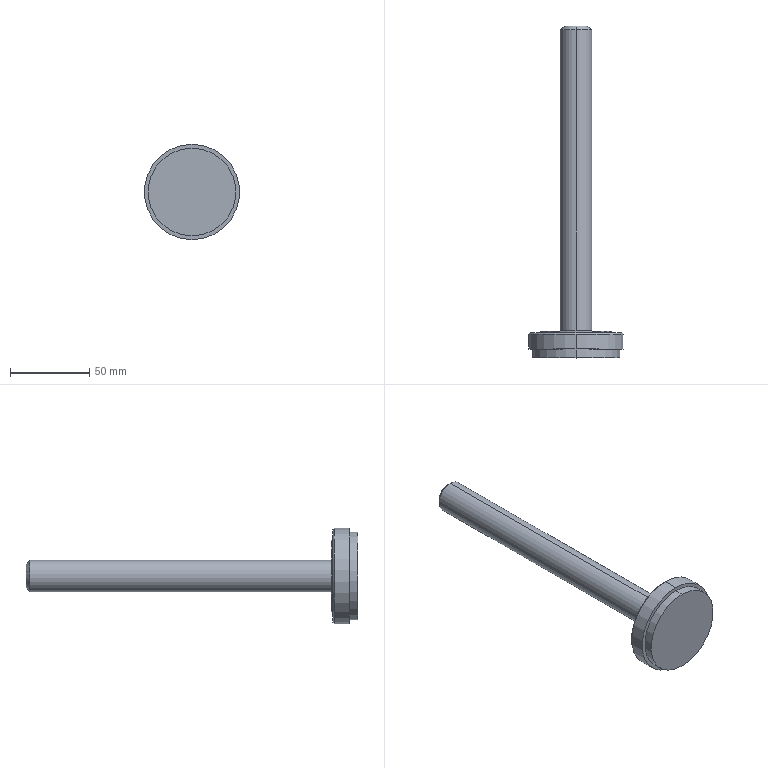Part | STEP file | SceondD-B3-20-180 | 1 solid | 17 faces | box 60.3 x 210 x 60.3 mm | volume 105197 mm3 | cylinder 8 | plane 5 | cone 4 | commonest cylinder face diameters 20 x2 45 x2 55.5 x2 60.3 x2
STEP:
#1=CARTESIAN_POINT('',(0.,0.,27.75));
#2=VERTEX_POINT('',#1);
#3=CARTESIAN_POINT('',(0.,0.,-27.75));
#4=VERTEX_POINT('',#3);
#5=CARTESIAN_POINT('',(0.,0.,0.));
#6=DIRECTION('',(0.,1.,0.));
#7=DIRECTION('',(0.,0.,1.));
#8=AXIS2_PLACEMENT_3D('',#5,#6,#7);
#9=CIRCLE('',#8,27.75);
#10=EDGE_CURVE('',#2,#4,#9,.T.);
#11=ORIENTED_EDGE('',*,*,#10,.T.);
#12=CARTESIAN_POINT('',(0.,5.6,-27.75));
#13=VERTEX_POINT('',#12);
#14=CARTESIAN_POINT('',(0.,210.,-27.75));
#15=DIRECTION('',(0.,1.,0.));
#16=VECTOR('',#15,1000.);
#17=LINE('',#14,#16);
#18=EDGE_CURVE('',#4,#13,#17,.T.);
#19=ORIENTED_EDGE('',*,*,#18,.T.);
#20=CARTESIAN_POINT('',(0.,5.6,27.75));
#21=VERTEX_POINT('',#20);
#22=CARTESIAN_POINT('',(0.,5.6,0.));
#23=DIRECTION('',(0.,1.,0.));
#24=DIRECTION('',(0.,0.,1.));
#25=AXIS2_PLACEMENT_3D('',#22,#23,#24);
#26=CIRCLE('',#25,27.75);
#27=EDGE_CURVE('',#21,#13,#26,.T.);
#28=ORIENTED_EDGE('',*,*,#27,.F.);
#29=CARTESIAN_POINT('',(0.,210.,27.75));
#30=DIRECTION('',(0.,1.,0.));
#31=VECTOR('',#30,1000.);
#32=LINE('',#29,#31);
#33=EDGE_CURVE('',#2,#21,#32,.T.);
#34=ORIENTED_EDGE('',*,*,#33,.F.);
#35=EDGE_LOOP('',(#11,#19,#28,#34));
#36=FACE_OUTER_BOUND('',#35,.T.);
#37=CARTESIAN_POINT('',(0.,210.,0.));
#38=DIRECTION('',(0.,1.,0.));
#39=DIRECTION('',(0.,0.,1.));
#40=AXIS2_PLACEMENT_3D('',#37,#38,#39);
#41=CYLINDRICAL_SURFACE('',#40,27.75);
#42=ADVANCED_FACE('',(#36),#41,.T.);
#43=CARTESIAN_POINT('',(0.,5.6,30.15));
#44=VERTEX_POINT('',#43);
#45=CARTESIAN_POINT('',(0.,5.6,-30.15));
#46=VERTEX_POINT('',#45);
#47=CARTESIAN_POINT('',(0.,5.6,0.));
#48=DIRECTION('',(0.,1.,0.));
#49=DIRECTION('',(0.,0.,1.));
#50=AXIS2_PLACEMENT_3D('',#47,#48,#49);
#51=CIRCLE('',#50,30.15);
#52=EDGE_CURVE('',#44,#46,#51,.T.);
#53=ORIENTED_EDGE('',*,*,#52,.T.);
#54=CARTESIAN_POINT('',(0.,15.,-30.15));
#55=VERTEX_POINT('',#54);
#56=CARTESIAN_POINT('',(0.,210.,-30.15));
#57=DIRECTION('',(0.,1.,0.));
#58=VECTOR('',#57,1000.);
#59=LINE('',#56,#58);
#60=EDGE_CURVE('',#46,#55,#59,.T.);
#61=ORIENTED_EDGE('',*,*,#60,.T.);
#62=CARTESIAN_POINT('',(0.,15.,30.15));
#63=VERTEX_POINT('',#62);
#64=CARTESIAN_POINT('',(0.,15.,0.));
#65=DIRECTION('',(0.,1.,0.));
#66=DIRECTION('',(0.,0.,1.));
#67=AXIS2_PLACEMENT_3D('',#64,#65,#66);
#68=CIRCLE('',#67,30.15);
#69=EDGE_CURVE('',#63,#55,#68,.T.);
#70=ORIENTED_EDGE('',*,*,#69,.F.);
#71=CARTESIAN_POINT('',(0.,210.,30.15));
#72=DIRECTION('',(0.,1.,0.));
#73=VECTOR('',#72,1000.);
#74=LINE('',#71,#73);
#75=EDGE_CURVE('',#44,#63,#74,.T.);
#76=ORIENTED_EDGE('',*,*,#75,.F.);
#77=EDGE_LOOP('',(#53,#61,#70,#76));
#78=FACE_OUTER_BOUND('',#77,.T.);
#79=CARTESIAN_POINT('',(0.,210.,0.));
#80=DIRECTION('',(0.,1.,0.));
#81=DIRECTION('',(0.,0.,1.));
#82=AXIS2_PLACEMENT_3D('',#79,#80,#81);
#83=CYLINDRICAL_SURFACE('',#82,30.15);
#84=ADVANCED_FACE('',(#78),#83,.T.);
#85=CARTESIAN_POINT('',(0.,16.,29.15));
#86=VERTEX_POINT('',#85);
#87=CARTESIAN_POINT('',(0.,16.,-29.15));
#88=VERTEX_POINT('',#87);
#89=CARTESIAN_POINT('',(0.,16.,0.));
#90=DIRECTION('',(0.,1.,0.));
#91=DIRECTION('',(0.,0.,1.));
#92=AXIS2_PLACEMENT_3D('',#89,#90,#91);
#93=CIRCLE('',#92,29.15);
#94=EDGE_CURVE('',#86,#88,#93,.T.);
#95=ORIENTED_EDGE('',*,*,#94,.F.);
#96=CARTESIAN_POINT('',(0.,16.,29.15));
#97=DIRECTION('',(0.,-0.7071,0.7071));
#98=VECTOR('',#97,1000.);
#99=LINE('',#96,#98);
#100=EDGE_CURVE('',#86,#63,#99,.T.);
#101=ORIENTED_EDGE('',*,*,#100,.T.);
#102=ORIENTED_EDGE('',*,*,#69,.T.);
#103=CARTESIAN_POINT('',(0.,16.,-29.15));
#104=DIRECTION('',(0.,-0.7071,-0.7071));
#105=VECTOR('',#104,1000.);
#106=LINE('',#103,#105);
#107=EDGE_CURVE('',#88,#55,#106,.T.);
#108=ORIENTED_EDGE('',*,*,#107,.F.);
#109=EDGE_LOOP('',(#95,#101,#102,#108));
#110=FACE_OUTER_BOUND('',#109,.T.);
#111=CARTESIAN_POINT('',(0.,16.,0.));
#112=DIRECTION('',(0.,-1.,0.));
#113=DIRECTION('',(0.,0.,-1.));
#114=AXIS2_PLACEMENT_3D('',#111,#112,#113);
#115=CONICAL_SURFACE('',#114,29.15,0.7854);
#116=ADVANCED_FACE('',(#110),#115,.T.);
#117=CARTESIAN_POINT('',(0.,16.,22.5));
#118=VERTEX_POINT('',#117);
#119=CARTESIAN_POINT('',(0.,16.,-22.5));
#120=VERTEX_POINT('',#119);
#121=CARTESIAN_POINT('',(0.,16.,0.));
#122=DIRECTION('',(0.,1.,0.));
#123=DIRECTION('',(0.,0.,1.));
#124=AXIS2_PLACEMENT_3D('',#121,#122,#123);
#125=CIRCLE('',#124,22.5);
#126=EDGE_CURVE('',#118,#120,#125,.T.);
#127=ORIENTED_EDGE('',*,*,#126,.T.);
#128=CARTESIAN_POINT('',(0.,17.,-22.5));
#129=VERTEX_POINT('',#128);
#130=CARTESIAN_POINT('',(0.,210.,-22.5));
#131=DIRECTION('',(0.,1.,0.));
#132=VECTOR('',#131,1000.);
#133=LINE('',#130,#132);
#134=EDGE_CURVE('',#120,#129,#133,.T.);
#135=ORIENTED_EDGE('',*,*,#134,.T.);
#136=CARTESIAN_POINT('',(0.,17.,22.5));
#137=VERTEX_POINT('',#136);
#138=CARTESIAN_POINT('',(0.,17.,0.));
#139=DIRECTION('',(0.,1.,0.));
#140=DIRECTION('',(0.,0.,1.));
#141=AXIS2_PLACEMENT_3D('',#138,#139,#140);
#142=CIRCLE('',#141,22.5);
#143=EDGE_CURVE('',#137,#129,#142,.T.);
#144=ORIENTED_EDGE('',*,*,#143,.F.);
#145=CARTESIAN_POINT('',(0.,210.,22.5));
#146=DIRECTION('',(0.,1.,0.));
#147=VECTOR('',#146,1000.);
#148=LINE('',#145,#147);
#149=EDGE_CURVE('',#118,#137,#148,.T.);
#150=ORIENTED_EDGE('',*,*,#149,.F.);
#151=EDGE_LOOP('',(#127,#135,#144,#150));
#152=FACE_OUTER_BOUND('',#151,.T.);
#153=CARTESIAN_POINT('',(0.,210.,0.));
#154=DIRECTION('',(0.,1.,0.));
#155=DIRECTION('',(0.,0.,1.));
#156=AXIS2_PLACEMENT_3D('',#153,#154,#155);
#157=CYLINDRICAL_SURFACE('',#156,22.5);
#158=ADVANCED_FACE('',(#152),#157,.T.);
#159=CARTESIAN_POINT('',(0.,17.,10.));
#160=VERTEX_POINT('',#159);
#161=CARTESIAN_POINT('',(0.,17.,-10.));
#162=VERTEX_POINT('',#161);
#163=CARTESIAN_POINT('',(0.,17.,0.));
#164=DIRECTION('',(0.,1.,0.));
#165=DIRECTION('',(0.,0.,1.));
#166=AXIS2_PLACEMENT_3D('',#163,#164,#165);
#167=CIRCLE('',#166,10.);
#168=EDGE_CURVE('',#160,#162,#167,.T.);
#169=ORIENTED_EDGE('',*,*,#168,.T.);
#170=CARTESIAN_POINT('',(0.,207.5,-10.));
#171=VERTEX_POINT('',#170);
#172=CARTESIAN_POINT('',(0.,210.,-10.));
#173=DIRECTION('',(0.,1.,0.));
#174=VECTOR('',#173,1000.);
#175=LINE('',#172,#174);
#176=EDGE_CURVE('',#162,#171,#175,.T.);
#177=ORIENTED_EDGE('',*,*,#176,.T.);
#178=CARTESIAN_POINT('',(0.,207.5,10.));
#179=VERTEX_POINT('',#178);
#180=CARTESIAN_POINT('',(0.,207.5,0.));
#181=DIRECTION('',(0.,1.,0.));
#182=DIRECTION('',(0.,0.,1.));
#183=AXIS2_PLACEMENT_3D('',#180,#181,#182);
#184=CIRCLE('',#183,10.);
#185=EDGE_CURVE('',#179,#171,#184,.T.);
#186=ORIENTED_EDGE('',*,*,#185,.F.);
#187=CARTESIAN_POINT('',(0.,210.,10.));
#188=DIRECTION('',(0.,1.,0.));
#189=VECTOR('',#188,1000.);
#190=LINE('',#187,#189);
#191=EDGE_CURVE('',#160,#179,#190,.T.);
#192=ORIENTED_EDGE('',*,*,#191,.F.);
#193=EDGE_LOOP('',(#169,#177,#186,#192));
#194=FACE_OUTER_BOUND('',#193,.T.);
#195=CARTESIAN_POINT('',(0.,210.,0.));
#196=DIRECTION('',(0.,1.,0.));
#197=DIRECTION('',(0.,0.,1.));
#198=AXIS2_PLACEMENT_3D('',#195,#196,#197);
#199=CYLINDRICAL_SURFACE('',#198,10.);
#200=ADVANCED_FACE('',(#194),#199,.T.);
#201=CARTESIAN_POINT('',(0.,210.,7.5));
#202=VERTEX_POINT('',#201);
#203=CARTESIAN_POINT('',(0.,210.,-7.5));
#204=VERTEX_POINT('',#203);
#205=CARTESIAN_POINT('',(0.,210.,0.));
#206=DIRECTION('',(0.,1.,0.));
#207=DIRECTION('',(0.,0.,1.));
#208=AXIS2_PLACEMENT_3D('',#205,#206,#207);
#209=CIRCLE('',#208,7.5);
#210=EDGE_CURVE('',#202,#204,#209,.T.);
#211=ORIENTED_EDGE('',*,*,#210,.F.);
#212=CARTESIAN_POINT('',(0.,210.,7.5));
#213=DIRECTION('',(0.,-0.7071,0.7071));
#214=VECTOR('',#213,1000.);
#215=LINE('',#212,#214);
#216=EDGE_CURVE('',#202,#179,#215,.T.);
#217=ORIENTED_EDGE('',*,*,#216,.T.);
#218=ORIENTED_EDGE('',*,*,#185,.T.);
#219=CARTESIAN_POINT('',(0.,210.,-7.5));
#220=DIRECTION('',(0.,-0.7071,-0.7071));
#221=VECTOR('',#220,1000.);
#222=LINE('',#219,#221);
#223=EDGE_CURVE('',#204,#171,#222,.T.);
#224=ORIENTED_EDGE('',*,*,#223,.F.);
#225=EDGE_LOOP('',(#211,#217,#218,#224));
#226=FACE_OUTER_BOUND('',#225,.T.);
#227=CARTESIAN_POINT('',(0.,210.,0.));
#228=DIRECTION('',(0.,-1.,0.));
#229=DIRECTION('',(0.,0.,-1.));
#230=AXIS2_PLACEMENT_3D('',#227,#228,#229);
#231=CONICAL_SURFACE('',#230,7.5,0.7854);
#232=ADVANCED_FACE('',(#226),#231,.T.);
#233=ORIENTED_EDGE('',*,*,#216,.F.);
#234=CARTESIAN_POINT('',(0.,210.,0.));
#235=DIRECTION('',(0.,1.,0.));
#236=DIRECTION('',(0.,0.,1.));
#237=AXIS2_PLACEMENT_3D('',#234,#235,#236);
#238=CIRCLE('',#237,7.5);
#239=EDGE_CURVE('',#204,#202,#238,.T.);
#240=ORIENTED_EDGE('',*,*,#239,.F.);
#241=ORIENTED_EDGE('',*,*,#223,.T.);
#242=CARTESIAN_POINT('',(0.,207.5,0.));
#243=DIRECTION('',(0.,1.,0.));
#244=DIRECTION('',(0.,0.,1.));
#245=AXIS2_PLACEMENT_3D('',#242,#243,#244);
#246=CIRCLE('',#245,10.);
#247=EDGE_CURVE('',#171,#179,#246,.T.);
#248=ORIENTED_EDGE('',*,*,#247,.T.);
#249=EDGE_LOOP('',(#233,#240,#241,#248));
#250=FACE_OUTER_BOUND('',#249,.T.);
#251=CARTESIAN_POINT('',(0.,210.,0.));
#252=DIRECTION('',(0.,-1.,0.));
#253=DIRECTION('',(0.,0.,-1.));
#254=AXIS2_PLACEMENT_3D('',#251,#252,#253);
#255=CONICAL_SURFACE('',#254,7.5,0.7854);
#256=ADVANCED_FACE('',(#250),#255,.T.);
#257=ORIENTED_EDGE('',*,*,#176,.F.);
#258=CARTESIAN_POINT('',(0.,17.,0.));
#259=DIRECTION('',(0.,1.,0.));
#260=DIRECTION('',(0.,0.,1.));
#261=AXIS2_PLACEMENT_3D('',#258,#259,#260);
#262=CIRCLE('',#261,10.);
#263=EDGE_CURVE('',#162,#160,#262,.T.);
#264=ORIENTED_EDGE('',*,*,#263,.T.);
#265=ORIENTED_EDGE('',*,*,#191,.T.);
#266=ORIENTED_EDGE('',*,*,#247,.F.);
#267=EDGE_LOOP('',(#257,#264,#265,#266));
#268=FACE_OUTER_BOUND('',#267,.T.);
#269=CARTESIAN_POINT('',(0.,210.,0.));
#270=DIRECTION('',(0.,1.,0.));
#271=DIRECTION('',(0.,0.,1.));
#272=AXIS2_PLACEMENT_3D('',#269,#270,#271);
#273=CYLINDRICAL_SURFACE('',#272,10.);
#274=ADVANCED_FACE('',(#268),#273,.T.);
#275=ORIENTED_EDGE('',*,*,#143,.T.);
#276=CARTESIAN_POINT('',(0.,17.,0.));
#277=DIRECTION('',(0.,1.,0.));
#278=DIRECTION('',(0.,0.,1.));
#279=AXIS2_PLACEMENT_3D('',#276,#277,#278);
#280=CIRCLE('',#279,22.5);
#281=EDGE_CURVE('',#129,#137,#280,.T.);
#282=ORIENTED_EDGE('',*,*,#281,.T.);
#283=EDGE_LOOP('',(#275,#282));
#284=FACE_OUTER_BOUND('',#283,.T.);
#285=ORIENTED_EDGE('',*,*,#168,.F.);
#286=ORIENTED_EDGE('',*,*,#263,.F.);
#287=EDGE_LOOP('',(#285,#286));
#288=FACE_BOUND('',#287,.T.);
#289=CARTESIAN_POINT('',(-22.5,17.,0.));
#290=DIRECTION('',(0.,1.,0.));
#291=DIRECTION('',(0.,0.,1.));
#292=AXIS2_PLACEMENT_3D('',#289,#290,#291);
#293=PLANE('',#292);
#294=ADVANCED_FACE('',(#284,#288),#293,.T.);
#295=ORIENTED_EDGE('',*,*,#134,.F.);
#296=CARTESIAN_POINT('',(0.,16.,0.));
#297=DIRECTION('',(0.,1.,0.));
#298=DIRECTION('',(0.,0.,1.));
#299=AXIS2_PLACEMENT_3D('',#296,#297,#298);
#300=CIRCLE('',#299,22.5);
#301=EDGE_CURVE('',#120,#118,#300,.T.);
#302=ORIENTED_EDGE('',*,*,#301,.T.);
#303=ORIENTED_EDGE('',*,*,#149,.T.);
#304=ORIENTED_EDGE('',*,*,#281,.F.);
#305=EDGE_LOOP('',(#295,#302,#303,#304));
#306=FACE_OUTER_BOUND('',#305,.T.);
#307=CARTESIAN_POINT('',(0.,210.,0.));
#308=DIRECTION('',(0.,1.,0.));
#309=DIRECTION('',(0.,0.,1.));
#310=AXIS2_PLACEMENT_3D('',#307,#308,#309);
#311=CYLINDRICAL_SURFACE('',#310,22.5);
#312=ADVANCED_FACE('',(#306),#311,.T.);
#313=CARTESIAN_POINT('',(0.,16.,0.));
#314=DIRECTION('',(0.,1.,0.));
#315=DIRECTION('',(0.,0.,1.));
#316=AXIS2_PLACEMENT_3D('',#313,#314,#315);
#317=CIRCLE('',#316,29.15);
#318=EDGE_CURVE('',#88,#86,#317,.T.);
#319=ORIENTED_EDGE('',*,*,#318,.T.);
#320=ORIENTED_EDGE('',*,*,#94,.T.);
#321=EDGE_LOOP('',(#319,#320));
#322=FACE_OUTER_BOUND('',#321,.T.);
#323=ORIENTED_EDGE('',*,*,#126,.F.);
#324=ORIENTED_EDGE('',*,*,#301,.F.);
#325=EDGE_LOOP('',(#323,#324));
#326=FACE_BOUND('',#325,.T.);
#327=CARTESIAN_POINT('',(-29.15,16.,0.));
#328=DIRECTION('',(0.,1.,0.));
#329=DIRECTION('',(0.,0.,1.));
#330=AXIS2_PLACEMENT_3D('',#327,#328,#329);
#331=PLANE('',#330);
#332=ADVANCED_FACE('',(#322,#326),#331,.T.);
#333=ORIENTED_EDGE('',*,*,#100,.F.);
#334=ORIENTED_EDGE('',*,*,#318,.F.);
#335=ORIENTED_EDGE('',*,*,#107,.T.);
#336=CARTESIAN_POINT('',(0.,15.,0.));
#337=DIRECTION('',(0.,1.,0.));
#338=DIRECTION('',(0.,0.,1.));
#339=AXIS2_PLACEMENT_3D('',#336,#337,#338);
#340=CIRCLE('',#339,30.15);
#341=EDGE_CURVE('',#55,#63,#340,.T.);
#342=ORIENTED_EDGE('',*,*,#341,.T.);
#343=EDGE_LOOP('',(#333,#334,#335,#342));
#344=FACE_OUTER_BOUND('',#343,.T.);
#345=CARTESIAN_POINT('',(0.,16.,0.));
#346=DIRECTION('',(0.,-1.,0.));
#347=DIRECTION('',(0.,0.,-1.));
#348=AXIS2_PLACEMENT_3D('',#345,#346,#347);
#349=CONICAL_SURFACE('',#348,29.15,0.7854);
#350=ADVANCED_FACE('',(#344),#349,.T.);
#351=ORIENTED_EDGE('',*,*,#60,.F.);
#352=CARTESIAN_POINT('',(0.,5.6,0.));
#353=DIRECTION('',(0.,1.,0.));
#354=DIRECTION('',(0.,0.,1.));
#355=AXIS2_PLACEMENT_3D('',#352,#353,#354);
#356=CIRCLE('',#355,30.15);
#357=EDGE_CURVE('',#46,#44,#356,.T.);
#358=ORIENTED_EDGE('',*,*,#357,.T.);
#359=ORIENTED_EDGE('',*,*,#75,.T.);
#360=ORIENTED_EDGE('',*,*,#341,.F.);
#361=EDGE_LOOP('',(#351,#358,#359,#360));
#362=FACE_OUTER_BOUND('',#361,.T.);
#363=CARTESIAN_POINT('',(0.,210.,0.));
#364=DIRECTION('',(0.,1.,0.));
#365=DIRECTION('',(0.,0.,1.));
#366=AXIS2_PLACEMENT_3D('',#363,#364,#365);
#367=CYLINDRICAL_SURFACE('',#366,30.15);
#368=ADVANCED_FACE('',(#362),#367,.T.);
#369=ORIENTED_EDGE('',*,*,#27,.T.);
#370=CARTESIAN_POINT('',(0.,5.6,0.));
#371=DIRECTION('',(0.,1.,0.));
#372=DIRECTION('',(0.,0.,1.));
#373=AXIS2_PLACEMENT_3D('',#370,#371,#372);
#374=CIRCLE('',#373,27.75);
#375=EDGE_CURVE('',#13,#21,#374,.T.);
#376=ORIENTED_EDGE('',*,*,#375,.T.);
#377=EDGE_LOOP('',(#369,#376));
#378=FACE_BOUND('',#377,.T.);
#379=ORIENTED_EDGE('',*,*,#52,.F.);
#380=ORIENTED_EDGE('',*,*,#357,.F.);
#381=EDGE_LOOP('',(#379,#380));
#382=FACE_OUTER_BOUND('',#381,.T.);
#383=CARTESIAN_POINT('',(-30.15,5.6,0.));
#384=DIRECTION('',(0.,-1.,0.));
#385=DIRECTION('',(0.,0.,-1.));
#386=AXIS2_PLACEMENT_3D('',#383,#384,#385);
#387=PLANE('',#386);
#388=ADVANCED_FACE('',(#378,#382),#387,.T.);
#389=ORIENTED_EDGE('',*,*,#18,.F.);
#390=CARTESIAN_POINT('',(0.,0.,0.));
#391=DIRECTION('',(0.,1.,0.));
#392=DIRECTION('',(0.,0.,1.));
#393=AXIS2_PLACEMENT_3D('',#390,#391,#392);
#394=CIRCLE('',#393,27.75);
#395=EDGE_CURVE('',#4,#2,#394,.T.);
#396=ORIENTED_EDGE('',*,*,#395,.T.);
#397=ORIENTED_EDGE('',*,*,#33,.T.);
#398=ORIENTED_EDGE('',*,*,#375,.F.);
#399=EDGE_LOOP('',(#389,#396,#397,#398));
#400=FACE_OUTER_BOUND('',#399,.T.);
#401=CARTESIAN_POINT('',(0.,210.,0.));
#402=DIRECTION('',(0.,1.,0.));
#403=DIRECTION('',(0.,0.,1.));
#404=AXIS2_PLACEMENT_3D('',#401,#402,#403);
#405=CYLINDRICAL_SURFACE('',#404,27.75);
#406=ADVANCED_FACE('',(#400),#405,.T.);
#407=ORIENTED_EDGE('',*,*,#10,.F.);
#408=ORIENTED_EDGE('',*,*,#395,.F.);
#409=EDGE_LOOP('',(#407,#408));
#410=FACE_OUTER_BOUND('',#409,.T.);
#411=CARTESIAN_POINT('',(0.,0.,0.));
#412=DIRECTION('',(0.,-1.,0.));
#413=DIRECTION('',(0.,0.,-1.));
#414=AXIS2_PLACEMENT_3D('',#411,#412,#413);
#415=PLANE('',#414);
#416=ADVANCED_FACE('',(#410),#415,.T.);
#417=ORIENTED_EDGE('',*,*,#239,.T.);
#418=ORIENTED_EDGE('',*,*,#210,.T.);
#419=EDGE_LOOP('',(#417,#418));
#420=FACE_OUTER_BOUND('',#419,.T.);
#421=CARTESIAN_POINT('',(0.,210.,0.));
#422=DIRECTION('',(0.,1.,0.));
#423=DIRECTION('',(0.,0.,1.));
#424=AXIS2_PLACEMENT_3D('',#421,#422,#423);
#425=PLANE('',#424);
#426=ADVANCED_FACE('',(#420),#425,.T.);
#427=CLOSED_SHELL('',(#42,#84,#116,#158,#200,#232,#256,#274,#294,#312,#332,#350,#368,#388,#406,#416,#426));
#428=MANIFOLD_SOLID_BREP('',#427);
#429=CARTESIAN_POINT('',(0.,0.,0.));
#430=DIRECTION('',(0.,0.,1.));
#431=DIRECTION('',(1.,0.,0.));
#432=AXIS2_PLACEMENT_3D('',#429,#430,#431);
#433=(LENGTH_UNIT()NAMED_UNIT(*)SI_UNIT(.MILLI.,.METRE.));
#434=UNCERTAINTY_MEASURE_WITH_UNIT(LENGTH_MEASURE(0.00001),#433,'','');
#435=(NAMED_UNIT(*)PLANE_ANGLE_UNIT()SI_UNIT($,.RADIAN.));
#436=(NAMED_UNIT(*)SI_UNIT($,.STERADIAN.)SOLID_ANGLE_UNIT());
#437=(GEOMETRIC_REPRESENTATION_CONTEXT(3)GLOBAL_UNCERTAINTY_ASSIGNED_CONTEXT((#434))GLOBAL_UNIT_ASSIGNED_CONTEXT((#433,#435,#436))REPRESENTATION_CONTEXT('',''));
#438=ADVANCED_BREP_SHAPE_REPRESENTATION('',(#428,#432),#437);